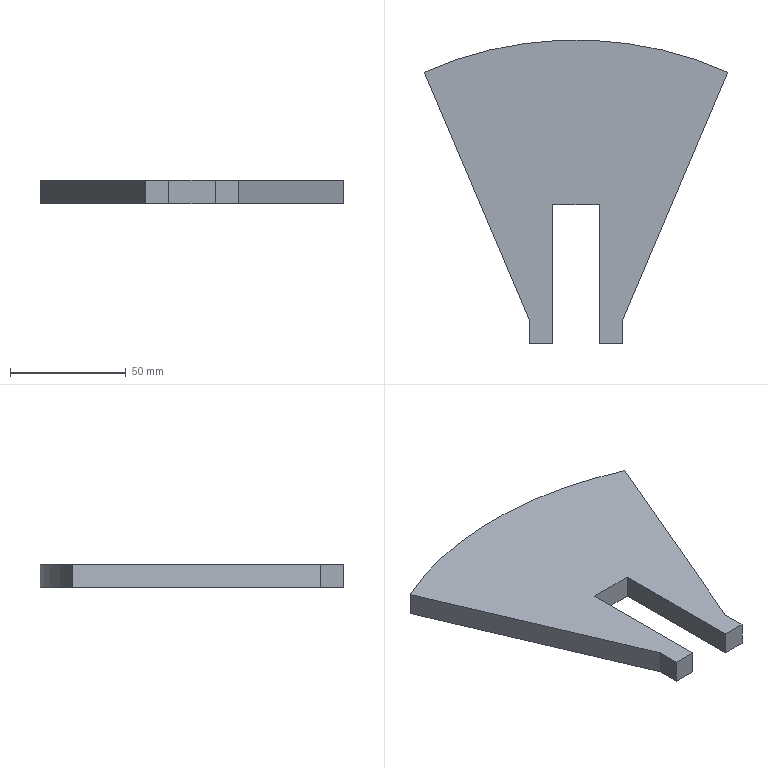Part | SolidWorks | features Extrusion 1, ICE 1 | 1 solid | 12 faces | box 130.916 x 131 x 10 mm | volume 95766 mm3 | plane 11 | cylinder 1 | commonest cylinder face diameters 322 x1
STEP:
#1=CARTESIAN_POINT('',(-20.,30.,-5.));
#2=VERTEX_POINT('',#1);
#3=CARTESIAN_POINT('',(-10.,30.,-5.));
#4=VERTEX_POINT('',#3);
#5=CARTESIAN_POINT('',(-20.,30.,-5.));
#6=DIRECTION('',(1.,0.,0.));
#7=VECTOR('',#6,1000.);
#8=LINE('',#5,#7);
#9=EDGE_CURVE('',#2,#4,#8,.T.);
#10=ORIENTED_EDGE('',*,*,#9,.T.);
#11=CARTESIAN_POINT('',(-10.,30.,5.));
#12=VERTEX_POINT('',#11);
#13=CARTESIAN_POINT('',(-10.,30.,5.));
#14=DIRECTION('',(0.,0.,1.));
#15=VECTOR('',#14,1000.);
#16=LINE('',#13,#15);
#17=EDGE_CURVE('',#4,#12,#16,.T.);
#18=ORIENTED_EDGE('',*,*,#17,.T.);
#19=CARTESIAN_POINT('',(-20.,30.,5.));
#20=VERTEX_POINT('',#19);
#21=CARTESIAN_POINT('',(-20.,30.,5.));
#22=DIRECTION('',(1.,0.,0.));
#23=VECTOR('',#22,1000.);
#24=LINE('',#21,#23);
#25=EDGE_CURVE('',#20,#12,#24,.T.);
#26=ORIENTED_EDGE('',*,*,#25,.F.);
#27=CARTESIAN_POINT('',(-20.,30.,5.));
#28=DIRECTION('',(0.,0.,-1.));
#29=VECTOR('',#28,1000.);
#30=LINE('',#27,#29);
#31=EDGE_CURVE('',#20,#2,#30,.T.);
#32=ORIENTED_EDGE('',*,*,#31,.T.);
#33=EDGE_LOOP('',(#10,#18,#26,#32));
#34=FACE_OUTER_BOUND('',#33,.T.);
#35=CARTESIAN_POINT('',(-20.,30.,5.));
#36=DIRECTION('',(0.,1.,0.));
#37=DIRECTION('',(-1.,0.,0.));
#38=AXIS2_PLACEMENT_3D('',#35,#36,#37);
#39=PLANE('',#38);
#40=ADVANCED_FACE('',(#34),#39,.F.);
#41=CARTESIAN_POINT('',(65.458,147.093,-5.));
#42=VERTEX_POINT('',#41);
#43=CARTESIAN_POINT('',(-65.458,147.093,-5.));
#44=VERTEX_POINT('',#43);
#45=CARTESIAN_POINT('',(0.,0.,-5.));
#46=DIRECTION('',(0.,0.,1.));
#47=DIRECTION('',(1.,0.,0.));
#48=AXIS2_PLACEMENT_3D('',#45,#46,#47);
#49=CIRCLE('',#48,161.);
#50=EDGE_CURVE('',#42,#44,#49,.T.);
#51=ORIENTED_EDGE('',*,*,#50,.T.);
#52=CARTESIAN_POINT('',(-65.458,147.093,5.));
#53=VERTEX_POINT('',#52);
#54=CARTESIAN_POINT('',(-65.458,147.093,5.));
#55=DIRECTION('',(0.,0.,-1.));
#56=VECTOR('',#55,1000.);
#57=LINE('',#54,#56);
#58=EDGE_CURVE('',#53,#44,#57,.T.);
#59=ORIENTED_EDGE('',*,*,#58,.F.);
#60=CARTESIAN_POINT('',(65.458,147.093,5.));
#61=VERTEX_POINT('',#60);
#62=CARTESIAN_POINT('',(0.,0.,5.));
#63=DIRECTION('',(0.,0.,1.));
#64=DIRECTION('',(1.,0.,0.));
#65=AXIS2_PLACEMENT_3D('',#62,#63,#64);
#66=CIRCLE('',#65,161.);
#67=EDGE_CURVE('',#61,#53,#66,.T.);
#68=ORIENTED_EDGE('',*,*,#67,.F.);
#69=CARTESIAN_POINT('',(65.458,147.093,5.));
#70=DIRECTION('',(0.,0.,-1.));
#71=VECTOR('',#70,1000.);
#72=LINE('',#69,#71);
#73=EDGE_CURVE('',#61,#42,#72,.T.);
#74=ORIENTED_EDGE('',*,*,#73,.T.);
#75=EDGE_LOOP('',(#51,#59,#68,#74));
#76=FACE_OUTER_BOUND('',#75,.T.);
#77=CARTESIAN_POINT('',(0.,0.,5.));
#78=DIRECTION('',(0.,0.,-1.));
#79=DIRECTION('',(-1.,0.,0.));
#80=AXIS2_PLACEMENT_3D('',#77,#78,#79);
#81=CYLINDRICAL_SURFACE('',#80,161.);
#82=ADVANCED_FACE('',(#76),#81,.T.);
#83=CARTESIAN_POINT('',(-20.,40.,-5.));
#84=VERTEX_POINT('',#83);
#85=CARTESIAN_POINT('',(-65.458,147.093,-5.));
#86=DIRECTION('',(0.3907,-0.9205,0.));
#87=VECTOR('',#86,1000.);
#88=LINE('',#85,#87);
#89=EDGE_CURVE('',#44,#84,#88,.T.);
#90=ORIENTED_EDGE('',*,*,#89,.T.);
#91=CARTESIAN_POINT('',(-20.,40.,5.));
#92=VERTEX_POINT('',#91);
#93=CARTESIAN_POINT('',(-20.,40.,5.));
#94=DIRECTION('',(0.,0.,-1.));
#95=VECTOR('',#94,1000.);
#96=LINE('',#93,#95);
#97=EDGE_CURVE('',#92,#84,#96,.T.);
#98=ORIENTED_EDGE('',*,*,#97,.F.);
#99=CARTESIAN_POINT('',(-65.458,147.093,5.));
#100=DIRECTION('',(0.3907,-0.9205,0.));
#101=VECTOR('',#100,1000.);
#102=LINE('',#99,#101);
#103=EDGE_CURVE('',#53,#92,#102,.T.);
#104=ORIENTED_EDGE('',*,*,#103,.F.);
#105=ORIENTED_EDGE('',*,*,#58,.T.);
#106=EDGE_LOOP('',(#90,#98,#104,#105));
#107=FACE_OUTER_BOUND('',#106,.T.);
#108=CARTESIAN_POINT('',(-65.458,147.093,5.));
#109=DIRECTION('',(0.9205,0.3907,0.));
#110=DIRECTION('',(-0.3907,0.9205,0.));
#111=AXIS2_PLACEMENT_3D('',#108,#109,#110);
#112=PLANE('',#111);
#113=ADVANCED_FACE('',(#107),#112,.F.);
#114=CARTESIAN_POINT('',(-20.,40.,-5.));
#115=DIRECTION('',(0.,-1.,0.));
#116=VECTOR('',#115,1000.);
#117=LINE('',#114,#116);
#118=EDGE_CURVE('',#84,#2,#117,.T.);
#119=ORIENTED_EDGE('',*,*,#118,.T.);
#120=ORIENTED_EDGE('',*,*,#31,.F.);
#121=CARTESIAN_POINT('',(-20.,40.,5.));
#122=DIRECTION('',(0.,-1.,0.));
#123=VECTOR('',#122,1000.);
#124=LINE('',#121,#123);
#125=EDGE_CURVE('',#92,#20,#124,.T.);
#126=ORIENTED_EDGE('',*,*,#125,.F.);
#127=ORIENTED_EDGE('',*,*,#97,.T.);
#128=EDGE_LOOP('',(#119,#120,#126,#127));
#129=FACE_OUTER_BOUND('',#128,.T.);
#130=CARTESIAN_POINT('',(-20.,40.,5.));
#131=DIRECTION('',(1.,0.,0.));
#132=DIRECTION('',(0.,0.,-1.));
#133=AXIS2_PLACEMENT_3D('',#130,#131,#132);
#134=PLANE('',#133);
#135=ADVANCED_FACE('',(#129),#134,.F.);
#136=CARTESIAN_POINT('',(10.,30.,5.));
#137=VERTEX_POINT('',#136);
#138=CARTESIAN_POINT('',(20.,30.,5.));
#139=VERTEX_POINT('',#138);
#140=CARTESIAN_POINT('',(-20.,30.,5.));
#141=DIRECTION('',(1.,0.,0.));
#142=VECTOR('',#141,1000.);
#143=LINE('',#140,#142);
#144=EDGE_CURVE('',#137,#139,#143,.T.);
#145=ORIENTED_EDGE('',*,*,#144,.F.);
#146=CARTESIAN_POINT('',(10.,30.,-5.));
#147=VERTEX_POINT('',#146);
#148=CARTESIAN_POINT('',(10.,30.,5.));
#149=DIRECTION('',(0.,0.,-1.));
#150=VECTOR('',#149,1000.);
#151=LINE('',#148,#150);
#152=EDGE_CURVE('',#137,#147,#151,.T.);
#153=ORIENTED_EDGE('',*,*,#152,.T.);
#154=CARTESIAN_POINT('',(20.,30.,-5.));
#155=VERTEX_POINT('',#154);
#156=CARTESIAN_POINT('',(-20.,30.,-5.));
#157=DIRECTION('',(1.,0.,0.));
#158=VECTOR('',#157,1000.);
#159=LINE('',#156,#158);
#160=EDGE_CURVE('',#147,#155,#159,.T.);
#161=ORIENTED_EDGE('',*,*,#160,.T.);
#162=CARTESIAN_POINT('',(20.,30.,5.));
#163=DIRECTION('',(0.,0.,-1.));
#164=VECTOR('',#163,1000.);
#165=LINE('',#162,#164);
#166=EDGE_CURVE('',#139,#155,#165,.T.);
#167=ORIENTED_EDGE('',*,*,#166,.F.);
#168=EDGE_LOOP('',(#145,#153,#161,#167));
#169=FACE_OUTER_BOUND('',#168,.T.);
#170=CARTESIAN_POINT('',(-20.,30.,5.));
#171=DIRECTION('',(0.,1.,0.));
#172=DIRECTION('',(-1.,0.,0.));
#173=AXIS2_PLACEMENT_3D('',#170,#171,#172);
#174=PLANE('',#173);
#175=ADVANCED_FACE('',(#169),#174,.F.);
#176=CARTESIAN_POINT('',(20.,40.,-5.));
#177=VERTEX_POINT('',#176);
#178=CARTESIAN_POINT('',(20.,30.,-5.));
#179=DIRECTION('',(0.,1.,0.));
#180=VECTOR('',#179,1000.);
#181=LINE('',#178,#180);
#182=EDGE_CURVE('',#155,#177,#181,.T.);
#183=ORIENTED_EDGE('',*,*,#182,.T.);
#184=CARTESIAN_POINT('',(20.,40.,5.));
#185=VERTEX_POINT('',#184);
#186=CARTESIAN_POINT('',(20.,40.,5.));
#187=DIRECTION('',(0.,0.,-1.));
#188=VECTOR('',#187,1000.);
#189=LINE('',#186,#188);
#190=EDGE_CURVE('',#185,#177,#189,.T.);
#191=ORIENTED_EDGE('',*,*,#190,.F.);
#192=CARTESIAN_POINT('',(20.,30.,5.));
#193=DIRECTION('',(0.,1.,0.));
#194=VECTOR('',#193,1000.);
#195=LINE('',#192,#194);
#196=EDGE_CURVE('',#139,#185,#195,.T.);
#197=ORIENTED_EDGE('',*,*,#196,.F.);
#198=ORIENTED_EDGE('',*,*,#166,.T.);
#199=EDGE_LOOP('',(#183,#191,#197,#198));
#200=FACE_OUTER_BOUND('',#199,.T.);
#201=CARTESIAN_POINT('',(20.,30.,5.));
#202=DIRECTION('',(-1.,0.,0.));
#203=DIRECTION('',(0.,0.,1.));
#204=AXIS2_PLACEMENT_3D('',#201,#202,#203);
#205=PLANE('',#204);
#206=ADVANCED_FACE('',(#200),#205,.F.);
#207=CARTESIAN_POINT('',(20.,40.,-5.));
#208=DIRECTION('',(0.3907,0.9205,0.));
#209=VECTOR('',#208,1000.);
#210=LINE('',#207,#209);
#211=EDGE_CURVE('',#177,#42,#210,.T.);
#212=ORIENTED_EDGE('',*,*,#211,.T.);
#213=ORIENTED_EDGE('',*,*,#73,.F.);
#214=CARTESIAN_POINT('',(20.,40.,5.));
#215=DIRECTION('',(0.3907,0.9205,0.));
#216=VECTOR('',#215,1000.);
#217=LINE('',#214,#216);
#218=EDGE_CURVE('',#185,#61,#217,.T.);
#219=ORIENTED_EDGE('',*,*,#218,.F.);
#220=ORIENTED_EDGE('',*,*,#190,.T.);
#221=EDGE_LOOP('',(#212,#213,#219,#220));
#222=FACE_OUTER_BOUND('',#221,.T.);
#223=CARTESIAN_POINT('',(20.,40.,5.));
#224=DIRECTION('',(-0.9205,0.3907,0.));
#225=DIRECTION('',(-0.3907,-0.9205,0.));
#226=AXIS2_PLACEMENT_3D('',#223,#224,#225);
#227=PLANE('',#226);
#228=ADVANCED_FACE('',(#222),#227,.F.);
#229=CARTESIAN_POINT('',(-10.,90.,5.));
#230=VERTEX_POINT('',#229);
#231=CARTESIAN_POINT('',(-10.,-30.,5.));
#232=DIRECTION('',(0.,-1.,0.));
#233=VECTOR('',#232,1000.);
#234=LINE('',#231,#233);
#235=EDGE_CURVE('',#230,#12,#234,.T.);
#236=ORIENTED_EDGE('',*,*,#235,.F.);
#237=CARTESIAN_POINT('',(10.,90.,5.));
#238=VERTEX_POINT('',#237);
#239=CARTESIAN_POINT('',(10.,90.,5.));
#240=DIRECTION('',(-1.,0.,0.));
#241=VECTOR('',#240,1000.);
#242=LINE('',#239,#241);
#243=EDGE_CURVE('',#238,#230,#242,.T.);
#244=ORIENTED_EDGE('',*,*,#243,.F.);
#245=CARTESIAN_POINT('',(10.,-30.,5.));
#246=DIRECTION('',(0.,1.,0.));
#247=VECTOR('',#246,1000.);
#248=LINE('',#245,#247);
#249=EDGE_CURVE('',#137,#238,#248,.T.);
#250=ORIENTED_EDGE('',*,*,#249,.F.);
#251=ORIENTED_EDGE('',*,*,#144,.T.);
#252=ORIENTED_EDGE('',*,*,#196,.T.);
#253=ORIENTED_EDGE('',*,*,#218,.T.);
#254=ORIENTED_EDGE('',*,*,#67,.T.);
#255=ORIENTED_EDGE('',*,*,#103,.T.);
#256=ORIENTED_EDGE('',*,*,#125,.T.);
#257=ORIENTED_EDGE('',*,*,#25,.T.);
#258=EDGE_LOOP('',(#236,#244,#250,#251,#252,#253,#254,#255,#256,#257));
#259=FACE_OUTER_BOUND('',#258,.T.);
#260=CARTESIAN_POINT('',(0.,0.,5.));
#261=DIRECTION('',(0.,0.,1.));
#262=DIRECTION('',(1.,0.,0.));
#263=AXIS2_PLACEMENT_3D('',#260,#261,#262);
#264=PLANE('',#263);
#265=ADVANCED_FACE('',(#259),#264,.T.);
#266=CARTESIAN_POINT('',(10.,90.,-5.));
#267=VERTEX_POINT('',#266);
#268=CARTESIAN_POINT('',(-10.,90.,-5.));
#269=VERTEX_POINT('',#268);
#270=CARTESIAN_POINT('',(10.,90.,-5.));
#271=DIRECTION('',(-1.,0.,0.));
#272=VECTOR('',#271,1000.);
#273=LINE('',#270,#272);
#274=EDGE_CURVE('',#267,#269,#273,.T.);
#275=ORIENTED_EDGE('',*,*,#274,.T.);
#276=CARTESIAN_POINT('',(-10.,-30.,-5.));
#277=DIRECTION('',(0.,-1.,0.));
#278=VECTOR('',#277,1000.);
#279=LINE('',#276,#278);
#280=EDGE_CURVE('',#269,#4,#279,.T.);
#281=ORIENTED_EDGE('',*,*,#280,.T.);
#282=ORIENTED_EDGE('',*,*,#9,.F.);
#283=ORIENTED_EDGE('',*,*,#118,.F.);
#284=ORIENTED_EDGE('',*,*,#89,.F.);
#285=ORIENTED_EDGE('',*,*,#50,.F.);
#286=ORIENTED_EDGE('',*,*,#211,.F.);
#287=ORIENTED_EDGE('',*,*,#182,.F.);
#288=ORIENTED_EDGE('',*,*,#160,.F.);
#289=CARTESIAN_POINT('',(10.,0.,-5.));
#290=DIRECTION('',(0.,1.,0.));
#291=VECTOR('',#290,1000.);
#292=LINE('',#289,#291);
#293=EDGE_CURVE('',#147,#267,#292,.T.);
#294=ORIENTED_EDGE('',*,*,#293,.T.);
#295=EDGE_LOOP('',(#275,#281,#282,#283,#284,#285,#286,#287,#288,#294));
#296=FACE_OUTER_BOUND('',#295,.T.);
#297=CARTESIAN_POINT('',(0.,0.,-5.));
#298=DIRECTION('',(0.,0.,1.));
#299=DIRECTION('',(1.,0.,0.));
#300=AXIS2_PLACEMENT_3D('',#297,#298,#299);
#301=PLANE('',#300);
#302=ADVANCED_FACE('',(#296),#301,.F.);
#303=ORIENTED_EDGE('',*,*,#280,.F.);
#304=CARTESIAN_POINT('',(-10.,90.,-5.));
#305=DIRECTION('',(0.,0.,1.));
#306=VECTOR('',#305,1000.);
#307=LINE('',#304,#306);
#308=EDGE_CURVE('',#269,#230,#307,.T.);
#309=ORIENTED_EDGE('',*,*,#308,.T.);
#310=ORIENTED_EDGE('',*,*,#235,.T.);
#311=ORIENTED_EDGE('',*,*,#17,.F.);
#312=EDGE_LOOP('',(#303,#309,#310,#311));
#313=FACE_OUTER_BOUND('',#312,.T.);
#314=CARTESIAN_POINT('',(-10.,-30.,-5.));
#315=DIRECTION('',(-1.,0.,0.));
#316=DIRECTION('',(0.,0.,1.));
#317=AXIS2_PLACEMENT_3D('',#314,#315,#316);
#318=PLANE('',#317);
#319=ADVANCED_FACE('',(#313),#318,.F.);
#320=ORIENTED_EDGE('',*,*,#249,.T.);
#321=CARTESIAN_POINT('',(10.,90.,-5.));
#322=DIRECTION('',(0.,0.,1.));
#323=VECTOR('',#322,1000.);
#324=LINE('',#321,#323);
#325=EDGE_CURVE('',#267,#238,#324,.T.);
#326=ORIENTED_EDGE('',*,*,#325,.F.);
#327=ORIENTED_EDGE('',*,*,#293,.F.);
#328=ORIENTED_EDGE('',*,*,#152,.F.);
#329=EDGE_LOOP('',(#320,#326,#327,#328));
#330=FACE_OUTER_BOUND('',#329,.T.);
#331=CARTESIAN_POINT('',(10.,-30.,-5.));
#332=DIRECTION('',(1.,0.,0.));
#333=DIRECTION('',(0.,0.,-1.));
#334=AXIS2_PLACEMENT_3D('',#331,#332,#333);
#335=PLANE('',#334);
#336=ADVANCED_FACE('',(#330),#335,.F.);
#337=ORIENTED_EDGE('',*,*,#243,.T.);
#338=ORIENTED_EDGE('',*,*,#308,.F.);
#339=ORIENTED_EDGE('',*,*,#274,.F.);
#340=ORIENTED_EDGE('',*,*,#325,.T.);
#341=EDGE_LOOP('',(#337,#338,#339,#340));
#342=FACE_OUTER_BOUND('',#341,.T.);
#343=CARTESIAN_POINT('',(10.,90.,-5.));
#344=DIRECTION('',(0.,1.,0.));
#345=DIRECTION('',(0.,0.,1.));
#346=AXIS2_PLACEMENT_3D('',#343,#344,#345);
#347=PLANE('',#346);
#348=ADVANCED_FACE('',(#342),#347,.F.);
#349=CLOSED_SHELL('',(#40,#82,#113,#135,#175,#206,#228,#265,#302,#319,#336,#348));
#350=MANIFOLD_SOLID_BREP('',#349);
#351=CARTESIAN_POINT('',(0.,0.,0.));
#352=DIRECTION('',(0.,0.,1.));
#353=DIRECTION('',(1.,0.,0.));
#354=AXIS2_PLACEMENT_3D('',#351,#352,#353);
#355=(LENGTH_UNIT()NAMED_UNIT(*)SI_UNIT(.MILLI.,.METRE.));
#356=UNCERTAINTY_MEASURE_WITH_UNIT(LENGTH_MEASURE(0.00001),#355,'','');
#357=(NAMED_UNIT(*)PLANE_ANGLE_UNIT()SI_UNIT($,.RADIAN.));
#358=(NAMED_UNIT(*)SI_UNIT($,.STERADIAN.)SOLID_ANGLE_UNIT());
#359=(GEOMETRIC_REPRESENTATION_CONTEXT(3)GLOBAL_UNCERTAINTY_ASSIGNED_CONTEXT((#356))GLOBAL_UNIT_ASSIGNED_CONTEXT((#355,#357,#358))REPRESENTATION_CONTEXT('',''));
#360=ADVANCED_BREP_SHAPE_REPRESENTATION('',(#350,#354),#359);